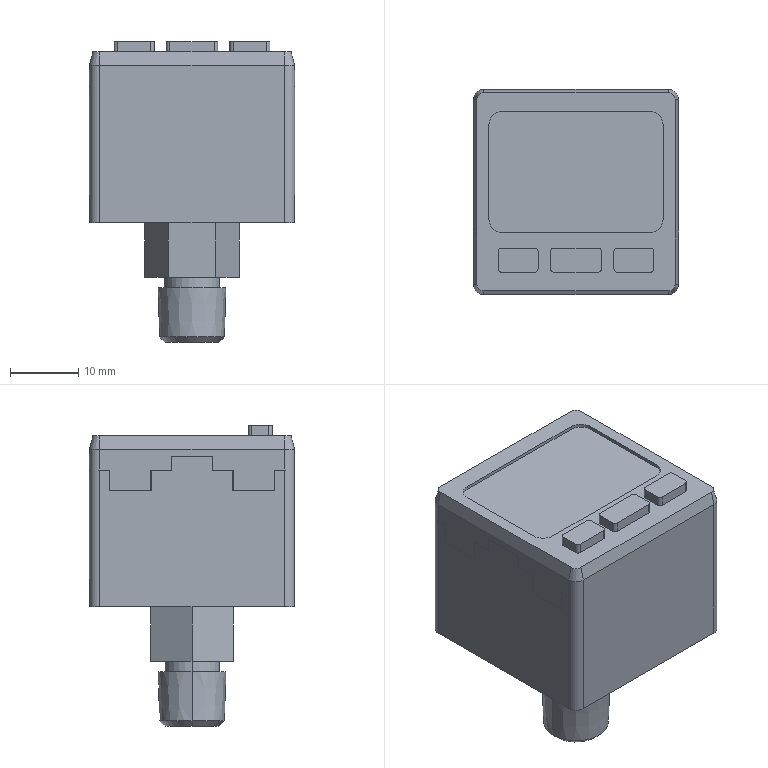Part | SolidWorks | features BaseBody 2 | 2 solids | 205 faces | box 30 x 30 x 44 mm | volume 22963 mm3 | plane 129 | cylinder 48 | cone 28 | commonest cylinder face diameters 1 x12 0.5 x10 3 x8 2.5 x4 2.6 x4 4 x4